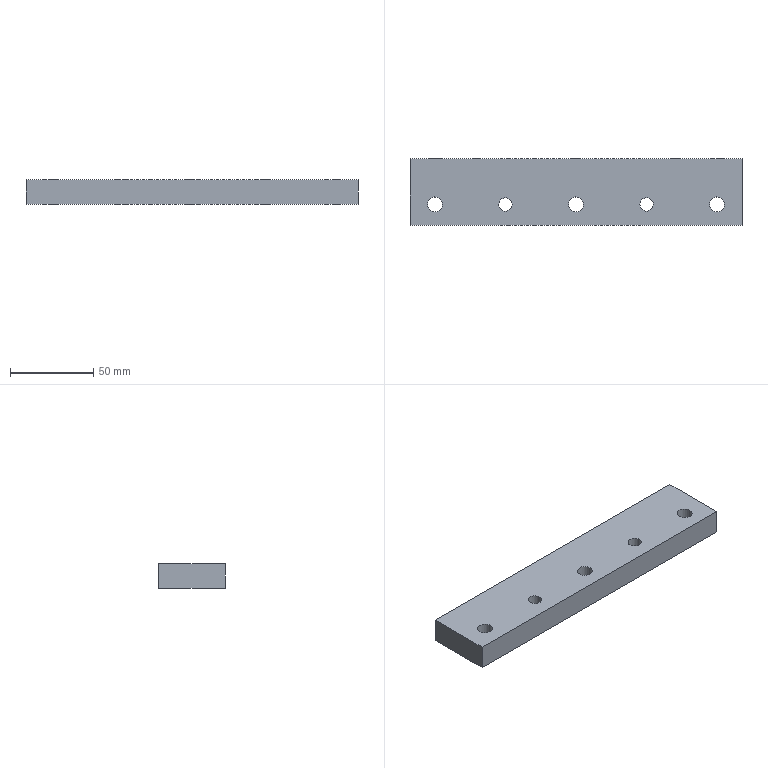Part | STEP file | SN10_002_007_SUPORTE | 1 solid | 21 faces | box 200 x 40 x 15 mm | volume 112375 mm3 | cylinder 10 | plane 6 | cone 5 | commonest cylinder face diameters 8 x4 4.917 x3 9 x3
STEP:
#1=CARTESIAN_POINT('',(0.,0.,0.));
#2=DIRECTION('',(0.,0.,1.));
#3=DIRECTION('',(1.,0.,0.));
#4=AXIS2_PLACEMENT_3D('',#1,#2,#3);
#5=CARTESIAN_POINT('',(-81.49,195.,59.418));
#6=VERTEX_POINT('',#5);
#7=CARTESIAN_POINT('',(-85.,195.,57.5));
#8=DIRECTION('',(0.,1.,0.));
#9=DIRECTION('',(1.,0.,0.));
#10=AXIS2_PLACEMENT_3D('',#7,#8,#9);
#11=CIRCLE('',#10,4.);
#12=CARTESIAN_POINT('',(-85.,193.268,57.5));
#13=DIRECTION('',(0.,1.,0.));
#14=DIRECTION('',(0.8776,0.,0.4794));
#15=AXIS2_PLACEMENT_3D('',#12,#13,#14);
#16=CONICAL_SURFACE('',#15,1.,1.047);
#17=CARTESIAN_POINT('',(-5.783,1.732));
#18=DIRECTION('',(1.,0.));
#19=VECTOR('',#18,1.);
#20=LINE('',#17,#19);
#21=(GEOMETRIC_REPRESENTATION_CONTEXT(2)PARAMETRIC_REPRESENTATION_CONTEXT()REPRESENTATION_CONTEXT('',''));
#22=DEFINITIONAL_REPRESENTATION('',(#20),#21);
#23=PCURVE('',#16,#22);
#24=CARTESIAN_POINT('',(-85.,214.9,57.5));
#25=DIRECTION('',(0.,-1.,0.));
#26=DIRECTION('',(0.8776,0.,0.4794));
#27=AXIS2_PLACEMENT_3D('',#24,#25,#26);
#28=CYLINDRICAL_SURFACE('',#27,4.);
#29=CARTESIAN_POINT('',(12.066,19.9));
#30=DIRECTION('',(-1.,0.));
#31=VECTOR('',#30,1.);
#32=LINE('',#29,#31);
#33=(GEOMETRIC_REPRESENTATION_CONTEXT(2)PARAMETRIC_REPRESENTATION_CONTEXT()REPRESENTATION_CONTEXT('',''));
#34=DEFINITIONAL_REPRESENTATION('',(#32),#33);
#35=PCURVE('',#28,#34);
#36=SURFACE_CURVE('',#11,(#23,#35),.PCURVE_S1.);
#37=EDGE_CURVE('',#6,#6,#36,.T.);
#38=ORIENTED_EDGE('',*,*,#37,.F.);
#39=CARTESIAN_POINT('',(-85.,192.691,57.5));
#40=VERTEX_POINT('',#39);
#41=CARTESIAN_POINT('',(-85.,192.691,57.5));
#42=CARTESIAN_POINT('',(-81.49,195.,59.418));
#43=B_SPLINE_CURVE_WITH_KNOTS('',1,(#41,#42),.UNSPECIFIED.,.F.,.F.,(2,2),(-1.155,3.464),.PIECEWISE_BEZIER_KNOTS.);
#44=CARTESIAN_POINT('',(0.,0.));
#45=DIRECTION('',(0.,1.));
#46=VECTOR('',#45,1.);
#47=LINE('',#44,#46);
#48=(GEOMETRIC_REPRESENTATION_CONTEXT(2)PARAMETRIC_REPRESENTATION_CONTEXT()REPRESENTATION_CONTEXT('',''));
#49=DEFINITIONAL_REPRESENTATION('',(#47),#48);
#50=PCURVE('',#16,#49);
#51=CARTESIAN_POINT('',(6.283,0.));
#52=DIRECTION('',(0.,1.));
#53=VECTOR('',#52,1.);
#54=LINE('',#51,#53);
#55=(GEOMETRIC_REPRESENTATION_CONTEXT(2)PARAMETRIC_REPRESENTATION_CONTEXT()REPRESENTATION_CONTEXT('',''));
#56=DEFINITIONAL_REPRESENTATION('',(#54),#55);
#57=PCURVE('',#16,#56);
#58=SEAM_CURVE('',#43,(#50,#57),.PCURVE_S1.);
#59=EDGE_CURVE('',#40,#6,#58,.T.);
#60=ORIENTED_EDGE('',*,*,#59,.F.);
#61=ORIENTED_EDGE('',*,*,#59,.T.);
#62=EDGE_LOOP('',(#38,#60,#61));
#63=FACE_BOUND('',#62,.F.);
#64=ADVANCED_FACE('',(#63),#16,.F.);
#65=CARTESIAN_POINT('',(-100.,215.,65.));
#66=VERTEX_POINT('',#65);
#67=CARTESIAN_POINT('',(100.,215.,65.));
#68=VERTEX_POINT('',#67);
#69=CARTESIAN_POINT('',(-100.,215.,65.));
#70=DIRECTION('',(1.,0.,0.));
#71=VECTOR('',#70,1.);
#72=LINE('',#69,#71);
#73=CARTESIAN_POINT('',(0.,175.,65.));
#74=DIRECTION('',(0.,0.,-1.));
#75=DIRECTION('',(-1.,0.,0.));
#76=AXIS2_PLACEMENT_3D('',#73,#74,#75);
#77=PLANE('',#76);
#78=CARTESIAN_POINT('',(100.,40.));
#79=DIRECTION('',(-1.,0.));
#80=VECTOR('',#79,1.);
#81=LINE('',#78,#80);
#82=(GEOMETRIC_REPRESENTATION_CONTEXT(2)PARAMETRIC_REPRESENTATION_CONTEXT()REPRESENTATION_CONTEXT('',''));
#83=DEFINITIONAL_REPRESENTATION('',(#81),#82);
#84=PCURVE('',#77,#83);
#85=CARTESIAN_POINT('',(0.,215.,65.));
#86=DIRECTION('',(0.,-1.,0.));
#87=DIRECTION('',(0.,0.,-1.));
#88=AXIS2_PLACEMENT_3D('',#85,#86,#87);
#89=PLANE('',#88);
#90=CARTESIAN_POINT('',(0.,-100.));
#91=DIRECTION('',(0.,1.));
#92=VECTOR('',#91,1.);
#93=LINE('',#90,#92);
#94=(GEOMETRIC_REPRESENTATION_CONTEXT(2)PARAMETRIC_REPRESENTATION_CONTEXT()REPRESENTATION_CONTEXT('',''));
#95=DEFINITIONAL_REPRESENTATION('',(#93),#94);
#96=PCURVE('',#89,#95);
#97=SURFACE_CURVE('',#72,(#84,#96),.PCURVE_S1.);
#98=EDGE_CURVE('',#66,#68,#97,.T.);
#99=ORIENTED_EDGE('',*,*,#98,.F.);
#100=CARTESIAN_POINT('',(-100.,175.,65.));
#101=VERTEX_POINT('',#100);
#102=CARTESIAN_POINT('',(-100.,175.,65.));
#103=DIRECTION('',(0.,1.,0.));
#104=VECTOR('',#103,1.);
#105=LINE('',#102,#104);
#106=CARTESIAN_POINT('',(100.,0.));
#107=DIRECTION('',(0.,1.));
#108=VECTOR('',#107,1.);
#109=LINE('',#106,#108);
#110=(GEOMETRIC_REPRESENTATION_CONTEXT(2)PARAMETRIC_REPRESENTATION_CONTEXT()REPRESENTATION_CONTEXT('',''));
#111=DEFINITIONAL_REPRESENTATION('',(#109),#110);
#112=PCURVE('',#77,#111);
#113=CARTESIAN_POINT('',(-100.,0.,0.));
#114=DIRECTION('',(1.,0.,0.));
#115=DIRECTION('',(0.,0.,-1.));
#116=AXIS2_PLACEMENT_3D('',#113,#114,#115);
#117=PLANE('',#116);
#118=CARTESIAN_POINT('',(-65.,175.));
#119=DIRECTION('',(0.,1.));
#120=VECTOR('',#119,1.);
#121=LINE('',#118,#120);
#122=(GEOMETRIC_REPRESENTATION_CONTEXT(2)PARAMETRIC_REPRESENTATION_CONTEXT()REPRESENTATION_CONTEXT('',''));
#123=DEFINITIONAL_REPRESENTATION('',(#121),#122);
#124=PCURVE('',#117,#123);
#125=SURFACE_CURVE('',#105,(#112,#124),.PCURVE_S1.);
#126=EDGE_CURVE('',#101,#66,#125,.T.);
#127=ORIENTED_EDGE('',*,*,#126,.F.);
#128=CARTESIAN_POINT('',(100.,175.,65.));
#129=VERTEX_POINT('',#128);
#130=CARTESIAN_POINT('',(-100.,175.,65.));
#131=DIRECTION('',(1.,0.,0.));
#132=VECTOR('',#131,1.);
#133=LINE('',#130,#132);
#134=CARTESIAN_POINT('',(100.,0.));
#135=DIRECTION('',(-1.,0.));
#136=VECTOR('',#135,1.);
#137=LINE('',#134,#136);
#138=(GEOMETRIC_REPRESENTATION_CONTEXT(2)PARAMETRIC_REPRESENTATION_CONTEXT()REPRESENTATION_CONTEXT('',''));
#139=DEFINITIONAL_REPRESENTATION('',(#137),#138);
#140=PCURVE('',#77,#139);
#141=CARTESIAN_POINT('',(0.,175.,50.));
#142=DIRECTION('',(0.,1.,0.));
#143=DIRECTION('',(0.,0.,1.));
#144=AXIS2_PLACEMENT_3D('',#141,#142,#143);
#145=PLANE('',#144);
#146=CARTESIAN_POINT('',(15.,-100.));
#147=DIRECTION('',(0.,1.));
#148=VECTOR('',#147,1.);
#149=LINE('',#146,#148);
#150=(GEOMETRIC_REPRESENTATION_CONTEXT(2)PARAMETRIC_REPRESENTATION_CONTEXT()REPRESENTATION_CONTEXT('',''));
#151=DEFINITIONAL_REPRESENTATION('',(#149),#150);
#152=PCURVE('',#145,#151);
#153=SURFACE_CURVE('',#133,(#140,#152),.PCURVE_S1.);
#154=EDGE_CURVE('',#101,#129,#153,.T.);
#155=ORIENTED_EDGE('',*,*,#154,.T.);
#156=CARTESIAN_POINT('',(100.,175.,65.));
#157=DIRECTION('',(0.,1.,0.));
#158=VECTOR('',#157,1.);
#159=LINE('',#156,#158);
#160=CARTESIAN_POINT('',(-100.,0.));
#161=DIRECTION('',(0.,1.));
#162=VECTOR('',#161,1.);
#163=LINE('',#160,#162);
#164=(GEOMETRIC_REPRESENTATION_CONTEXT(2)PARAMETRIC_REPRESENTATION_CONTEXT()REPRESENTATION_CONTEXT('',''));
#165=DEFINITIONAL_REPRESENTATION('',(#163),#164);
#166=PCURVE('',#77,#165);
#167=CARTESIAN_POINT('',(100.,0.,0.));
#168=DIRECTION('',(1.,0.,0.));
#169=DIRECTION('',(0.,0.,-1.));
#170=AXIS2_PLACEMENT_3D('',#167,#168,#169);
#171=PLANE('',#170);
#172=CARTESIAN_POINT('',(-65.,175.));
#173=DIRECTION('',(0.,1.));
#174=VECTOR('',#173,1.);
#175=LINE('',#172,#174);
#176=(GEOMETRIC_REPRESENTATION_CONTEXT(2)PARAMETRIC_REPRESENTATION_CONTEXT()REPRESENTATION_CONTEXT('',''));
#177=DEFINITIONAL_REPRESENTATION('',(#175),#176);
#178=PCURVE('',#171,#177);
#179=SURFACE_CURVE('',#159,(#166,#178),.PCURVE_S1.);
#180=EDGE_CURVE('',#129,#68,#179,.T.);
#181=ORIENTED_EDGE('',*,*,#180,.T.);
#182=EDGE_LOOP('',(#99,#127,#155,#181));
#183=FACE_BOUND('',#182,.T.);
#184=CARTESIAN_POINT('',(38.99,189.418,65.));
#185=VERTEX_POINT('',#184);
#186=CARTESIAN_POINT('',(42.5,187.5,65.));
#187=DIRECTION('',(0.,0.,-1.));
#188=DIRECTION('',(1.,0.,0.));
#189=AXIS2_PLACEMENT_3D('',#186,#187,#188);
#190=CIRCLE('',#189,4.);
#191=CARTESIAN_POINT('',(-42.5,12.5));
#192=DIRECTION('',(-1.,0.));
#193=AXIS2_PLACEMENT_2D('',#191,#192);
#194=CIRCLE('',#193,4.);
#195=(GEOMETRIC_REPRESENTATION_CONTEXT(2)PARAMETRIC_REPRESENTATION_CONTEXT()REPRESENTATION_CONTEXT('',''));
#196=DEFINITIONAL_REPRESENTATION('',(#194),#195);
#197=PCURVE('',#77,#196);
#198=CARTESIAN_POINT('',(42.5,187.5,64.9));
#199=DIRECTION('',(0.,0.,-1.));
#200=DIRECTION('',(0.8776,-0.4794,0.));
#201=AXIS2_PLACEMENT_3D('',#198,#199,#200);
#202=CYLINDRICAL_SURFACE('',#201,4.);
#203=CARTESIAN_POINT('',(-0.5,-0.1));
#204=DIRECTION('',(1.,0.));
#205=VECTOR('',#204,1.);
#206=LINE('',#203,#205);
#207=(GEOMETRIC_REPRESENTATION_CONTEXT(2)PARAMETRIC_REPRESENTATION_CONTEXT()REPRESENTATION_CONTEXT('',''));
#208=DEFINITIONAL_REPRESENTATION('',(#206),#207);
#209=PCURVE('',#202,#208);
#210=SURFACE_CURVE('',#190,(#197,#209),.PCURVE_S1.);
#211=EDGE_CURVE('',#185,#185,#210,.T.);
#212=ORIENTED_EDGE('',*,*,#211,.T.);
#213=EDGE_LOOP('',(#212));
#214=FACE_BOUND('',#213,.T.);
#215=CARTESIAN_POINT('',(-46.01,189.418,65.));
#216=VERTEX_POINT('',#215);
#217=CARTESIAN_POINT('',(-42.5,187.5,65.));
#218=DIRECTION('',(0.,0.,-1.));
#219=DIRECTION('',(1.,0.,0.));
#220=AXIS2_PLACEMENT_3D('',#217,#218,#219);
#221=CIRCLE('',#220,4.);
#222=CARTESIAN_POINT('',(42.5,12.5));
#223=DIRECTION('',(-1.,0.));
#224=AXIS2_PLACEMENT_2D('',#222,#223);
#225=CIRCLE('',#224,4.);
#226=(GEOMETRIC_REPRESENTATION_CONTEXT(2)PARAMETRIC_REPRESENTATION_CONTEXT()REPRESENTATION_CONTEXT('',''));
#227=DEFINITIONAL_REPRESENTATION('',(#225),#226);
#228=PCURVE('',#77,#227);
#229=CARTESIAN_POINT('',(-42.5,187.5,64.9));
#230=DIRECTION('',(0.,0.,-1.));
#231=DIRECTION('',(0.8776,-0.4794,0.));
#232=AXIS2_PLACEMENT_3D('',#229,#230,#231);
#233=CYLINDRICAL_SURFACE('',#232,4.);
#234=CARTESIAN_POINT('',(-0.5,-0.1));
#235=DIRECTION('',(1.,0.));
#236=VECTOR('',#235,1.);
#237=LINE('',#234,#236);
#238=(GEOMETRIC_REPRESENTATION_CONTEXT(2)PARAMETRIC_REPRESENTATION_CONTEXT()REPRESENTATION_CONTEXT('',''));
#239=DEFINITIONAL_REPRESENTATION('',(#237),#238);
#240=PCURVE('',#233,#239);
#241=SURFACE_CURVE('',#221,(#228,#240),.PCURVE_S1.);
#242=EDGE_CURVE('',#216,#216,#241,.T.);
#243=ORIENTED_EDGE('',*,*,#242,.T.);
#244=EDGE_LOOP('',(#243));
#245=FACE_BOUND('',#244,.T.);
#246=CARTESIAN_POINT('',(-88.949,189.657,65.));
#247=VERTEX_POINT('',#246);
#248=CARTESIAN_POINT('',(-85.,187.5,65.));
#249=DIRECTION('',(0.,0.,-1.));
#250=DIRECTION('',(1.,0.,0.));
#251=AXIS2_PLACEMENT_3D('',#248,#249,#250);
#252=CIRCLE('',#251,4.5);
#253=CARTESIAN_POINT('',(85.,12.5));
#254=DIRECTION('',(-1.,0.));
#255=AXIS2_PLACEMENT_2D('',#253,#254);
#256=CIRCLE('',#255,4.5);
#257=(GEOMETRIC_REPRESENTATION_CONTEXT(2)PARAMETRIC_REPRESENTATION_CONTEXT()REPRESENTATION_CONTEXT('',''));
#258=DEFINITIONAL_REPRESENTATION('',(#256),#257);
#259=PCURVE('',#77,#258);
#260=CARTESIAN_POINT('',(-85.,187.5,64.9));
#261=DIRECTION('',(0.,0.,-1.));
#262=DIRECTION('',(0.8776,-0.4794,0.));
#263=AXIS2_PLACEMENT_3D('',#260,#261,#262);
#264=CYLINDRICAL_SURFACE('',#263,4.5);
#265=CARTESIAN_POINT('',(-0.5,-0.1));
#266=DIRECTION('',(1.,0.));
#267=VECTOR('',#266,1.);
#268=LINE('',#265,#267);
#269=(GEOMETRIC_REPRESENTATION_CONTEXT(2)PARAMETRIC_REPRESENTATION_CONTEXT()REPRESENTATION_CONTEXT('',''));
#270=DEFINITIONAL_REPRESENTATION('',(#268),#269);
#271=PCURVE('',#264,#270);
#272=SURFACE_CURVE('',#252,(#259,#271),.PCURVE_S1.);
#273=EDGE_CURVE('',#247,#247,#272,.T.);
#274=ORIENTED_EDGE('',*,*,#273,.T.);
#275=EDGE_LOOP('',(#274));
#276=FACE_BOUND('',#275,.T.);
#277=CARTESIAN_POINT('',(-3.949,189.657,65.));
#278=VERTEX_POINT('',#277);
#279=CARTESIAN_POINT('',(0.,187.5,65.));
#280=DIRECTION('',(0.,0.,-1.));
#281=DIRECTION('',(1.,0.,0.));
#282=AXIS2_PLACEMENT_3D('',#279,#280,#281);
#283=CIRCLE('',#282,4.5);
#284=CARTESIAN_POINT('',(0.,12.5));
#285=DIRECTION('',(-1.,0.));
#286=AXIS2_PLACEMENT_2D('',#284,#285);
#287=CIRCLE('',#286,4.5);
#288=(GEOMETRIC_REPRESENTATION_CONTEXT(2)PARAMETRIC_REPRESENTATION_CONTEXT()REPRESENTATION_CONTEXT('',''));
#289=DEFINITIONAL_REPRESENTATION('',(#287),#288);
#290=PCURVE('',#77,#289);
#291=CARTESIAN_POINT('',(0.,187.5,64.9));
#292=DIRECTION('',(0.,0.,-1.));
#293=DIRECTION('',(0.8776,-0.4794,0.));
#294=AXIS2_PLACEMENT_3D('',#291,#292,#293);
#295=CYLINDRICAL_SURFACE('',#294,4.5);
#296=CARTESIAN_POINT('',(-0.5,-0.1));
#297=DIRECTION('',(1.,0.));
#298=VECTOR('',#297,1.);
#299=LINE('',#296,#298);
#300=(GEOMETRIC_REPRESENTATION_CONTEXT(2)PARAMETRIC_REPRESENTATION_CONTEXT()REPRESENTATION_CONTEXT('',''));
#301=DEFINITIONAL_REPRESENTATION('',(#299),#300);
#302=PCURVE('',#295,#301);
#303=SURFACE_CURVE('',#283,(#290,#302),.PCURVE_S1.);
#304=EDGE_CURVE('',#278,#278,#303,.T.);
#305=ORIENTED_EDGE('',*,*,#304,.T.);
#306=EDGE_LOOP('',(#305));
#307=FACE_BOUND('',#306,.T.);
#308=CARTESIAN_POINT('',(81.051,189.657,65.));
#309=VERTEX_POINT('',#308);
#310=CARTESIAN_POINT('',(85.,187.5,65.));
#311=DIRECTION('',(0.,0.,-1.));
#312=DIRECTION('',(1.,0.,0.));
#313=AXIS2_PLACEMENT_3D('',#310,#311,#312);
#314=CIRCLE('',#313,4.5);
#315=CARTESIAN_POINT('',(-85.,12.5));
#316=DIRECTION('',(-1.,0.));
#317=AXIS2_PLACEMENT_2D('',#315,#316);
#318=CIRCLE('',#317,4.5);
#319=(GEOMETRIC_REPRESENTATION_CONTEXT(2)PARAMETRIC_REPRESENTATION_CONTEXT()REPRESENTATION_CONTEXT('',''));
#320=DEFINITIONAL_REPRESENTATION('',(#318),#319);
#321=PCURVE('',#77,#320);
#322=CARTESIAN_POINT('',(85.,187.5,64.9));
#323=DIRECTION('',(0.,0.,-1.));
#324=DIRECTION('',(0.8776,-0.4794,0.));
#325=AXIS2_PLACEMENT_3D('',#322,#323,#324);
#326=CYLINDRICAL_SURFACE('',#325,4.5);
#327=CARTESIAN_POINT('',(-0.5,-0.1));
#328=DIRECTION('',(1.,0.));
#329=VECTOR('',#328,1.);
#330=LINE('',#327,#329);
#331=(GEOMETRIC_REPRESENTATION_CONTEXT(2)PARAMETRIC_REPRESENTATION_CONTEXT()REPRESENTATION_CONTEXT('',''));
#332=DEFINITIONAL_REPRESENTATION('',(#330),#331);
#333=PCURVE('',#326,#332);
#334=SURFACE_CURVE('',#314,(#321,#333),.PCURVE_S1.);
#335=EDGE_CURVE('',#309,#309,#334,.T.);
#336=ORIENTED_EDGE('',*,*,#335,.T.);
#337=EDGE_LOOP('',(#336));
#338=FACE_BOUND('',#337,.T.);
#339=ADVANCED_FACE('',(#183,#214,#245,#276,#307,#338),#77,.F.);
#340=CARTESIAN_POINT('',(-100.,215.,50.));
#341=VERTEX_POINT('',#340);
#342=CARTESIAN_POINT('',(-100.,215.,65.));
#343=DIRECTION('',(0.,0.,-1.));
#344=VECTOR('',#343,1.);
#345=LINE('',#342,#344);
#346=CARTESIAN_POINT('',(-65.,215.));
#347=DIRECTION('',(1.,0.));
#348=VECTOR('',#347,1.);
#349=LINE('',#346,#348);
#350=(GEOMETRIC_REPRESENTATION_CONTEXT(2)PARAMETRIC_REPRESENTATION_CONTEXT()REPRESENTATION_CONTEXT('',''));
#351=DEFINITIONAL_REPRESENTATION('',(#349),#350);
#352=PCURVE('',#117,#351);
#353=CARTESIAN_POINT('',(0.,-100.));
#354=DIRECTION('',(1.,0.));
#355=VECTOR('',#354,1.);
#356=LINE('',#353,#355);
#357=(GEOMETRIC_REPRESENTATION_CONTEXT(2)PARAMETRIC_REPRESENTATION_CONTEXT()REPRESENTATION_CONTEXT('',''));
#358=DEFINITIONAL_REPRESENTATION('',(#356),#357);
#359=PCURVE('',#89,#358);
#360=SURFACE_CURVE('',#345,(#352,#359),.PCURVE_S1.);
#361=EDGE_CURVE('',#66,#341,#360,.T.);
#362=ORIENTED_EDGE('',*,*,#361,.T.);
#363=CARTESIAN_POINT('',(-100.,175.,50.));
#364=VERTEX_POINT('',#363);
#365=CARTESIAN_POINT('',(-100.,215.,50.));
#366=DIRECTION('',(0.,-1.,0.));
#367=VECTOR('',#366,1.);
#368=LINE('',#365,#367);
#369=CARTESIAN_POINT('',(-50.,215.));
#370=DIRECTION('',(0.,-1.));
#371=VECTOR('',#370,1.);
#372=LINE('',#369,#371);
#373=(GEOMETRIC_REPRESENTATION_CONTEXT(2)PARAMETRIC_REPRESENTATION_CONTEXT()REPRESENTATION_CONTEXT('',''));
#374=DEFINITIONAL_REPRESENTATION('',(#372),#373);
#375=PCURVE('',#117,#374);
#376=CARTESIAN_POINT('',(0.,215.,50.));
#377=DIRECTION('',(0.,0.,1.));
#378=DIRECTION('',(1.,0.,0.));
#379=AXIS2_PLACEMENT_3D('',#376,#377,#378);
#380=PLANE('',#379);
#381=CARTESIAN_POINT('',(-100.,0.));
#382=DIRECTION('',(0.,-1.));
#383=VECTOR('',#382,1.);
#384=LINE('',#381,#383);
#385=(GEOMETRIC_REPRESENTATION_CONTEXT(2)PARAMETRIC_REPRESENTATION_CONTEXT()REPRESENTATION_CONTEXT('',''));
#386=DEFINITIONAL_REPRESENTATION('',(#384),#385);
#387=PCURVE('',#380,#386);
#388=SURFACE_CURVE('',#368,(#375,#387),.PCURVE_S1.);
#389=EDGE_CURVE('',#341,#364,#388,.T.);
#390=ORIENTED_EDGE('',*,*,#389,.T.);
#391=CARTESIAN_POINT('',(-100.,175.,50.));
#392=DIRECTION('',(0.,0.,1.));
#393=VECTOR('',#392,1.);
#394=LINE('',#391,#393);
#395=CARTESIAN_POINT('',(-50.,175.));
#396=DIRECTION('',(-1.,0.));
#397=VECTOR('',#396,1.);
#398=LINE('',#395,#397);
#399=(GEOMETRIC_REPRESENTATION_CONTEXT(2)PARAMETRIC_REPRESENTATION_CONTEXT()REPRESENTATION_CONTEXT('',''));
#400=DEFINITIONAL_REPRESENTATION('',(#398),#399);
#401=PCURVE('',#117,#400);
#402=CARTESIAN_POINT('',(0.,-100.));
#403=DIRECTION('',(1.,0.));
#404=VECTOR('',#403,1.);
#405=LINE('',#402,#404);
#406=(GEOMETRIC_REPRESENTATION_CONTEXT(2)PARAMETRIC_REPRESENTATION_CONTEXT()REPRESENTATION_CONTEXT('',''));
#407=DEFINITIONAL_REPRESENTATION('',(#405),#406);
#408=PCURVE('',#145,#407);
#409=SURFACE_CURVE('',#394,(#401,#408),.PCURVE_S1.);
#410=EDGE_CURVE('',#364,#101,#409,.T.);
#411=ORIENTED_EDGE('',*,*,#410,.T.);
#412=ORIENTED_EDGE('',*,*,#126,.T.);
#413=EDGE_LOOP('',(#362,#390,#411,#412));
#414=FACE_BOUND('',#413,.T.);
#415=ADVANCED_FACE('',(#414),#117,.F.);
#416=CARTESIAN_POINT('',(81.49,215.,55.582));
#417=VERTEX_POINT('',#416);
#418=CARTESIAN_POINT('',(85.,215.,57.5));
#419=DIRECTION('',(0.,-1.,0.));
#420=DIRECTION('',(1.,0.,0.));
#421=AXIS2_PLACEMENT_3D('',#418,#419,#420);
#422=CIRCLE('',#421,4.);
#423=CARTESIAN_POINT('',(85.,214.9,57.5));
#424=DIRECTION('',(0.,-1.,0.));
#425=DIRECTION('',(0.8776,0.,0.4794));
#426=AXIS2_PLACEMENT_3D('',#423,#424,#425);
#427=CYLINDRICAL_SURFACE('',#426,4.);
#428=CARTESIAN_POINT('',(-0.5,-0.1));
#429=DIRECTION('',(1.,0.));
#430=VECTOR('',#429,1.);
#431=LINE('',#428,#430);
#432=(GEOMETRIC_REPRESENTATION_CONTEXT(2)PARAMETRIC_REPRESENTATION_CONTEXT()REPRESENTATION_CONTEXT('',''));
#433=DEFINITIONAL_REPRESENTATION('',(#431),#432);
#434=PCURVE('',#427,#433);
#435=CARTESIAN_POINT('',(7.5,85.));
#436=DIRECTION('',(0.,1.));
#437=AXIS2_PLACEMENT_2D('',#435,#436);
#438=CIRCLE('',#437,4.);
#439=(GEOMETRIC_REPRESENTATION_CONTEXT(2)PARAMETRIC_REPRESENTATION_CONTEXT()REPRESENTATION_CONTEXT('',''));
#440=DEFINITIONAL_REPRESENTATION('',(#438),#439);
#441=PCURVE('',#89,#440);
#442=SURFACE_CURVE('',#422,(#434,#441),.PCURVE_S1.);
#443=EDGE_CURVE('',#417,#417,#442,.T.);
#444=ORIENTED_EDGE('',*,*,#443,.T.);
#445=CARTESIAN_POINT('',(81.49,195.,55.582));
#446=VERTEX_POINT('',#445);
#447=CARTESIAN_POINT('',(81.49,215.,55.582));
#448=CARTESIAN_POINT('',(81.49,195.,55.582));
#449=B_SPLINE_CURVE_WITH_KNOTS('',1,(#447,#448),.UNSPECIFIED.,.F.,.F.,(2,2),(-0.1,19.9),.PIECEWISE_BEZIER_KNOTS.);
#450=CARTESIAN_POINT('',(9.425,0.));
#451=DIRECTION('',(0.,1.));
#452=VECTOR('',#451,1.);
#453=LINE('',#450,#452);
#454=(GEOMETRIC_REPRESENTATION_CONTEXT(2)PARAMETRIC_REPRESENTATION_CONTEXT()REPRESENTATION_CONTEXT('',''));
#455=DEFINITIONAL_REPRESENTATION('',(#453),#454);
#456=PCURVE('',#427,#455);
#457=CARTESIAN_POINT('',(3.142,0.));
#458=DIRECTION('',(0.,1.));
#459=VECTOR('',#458,1.);
#460=LINE('',#457,#459);
#461=(GEOMETRIC_REPRESENTATION_CONTEXT(2)PARAMETRIC_REPRESENTATION_CONTEXT()REPRESENTATION_CONTEXT('',''));
#462=DEFINITIONAL_REPRESENTATION('',(#460),#461);
#463=PCURVE('',#427,#462);
#464=SEAM_CURVE('',#449,(#456,#463),.PCURVE_S1.);
#465=EDGE_CURVE('',#417,#446,#464,.T.);
#466=ORIENTED_EDGE('',*,*,#465,.T.);
#467=CARTESIAN_POINT('',(85.,195.,57.5));
#468=DIRECTION('',(0.,-1.,0.));
#469=DIRECTION('',(1.,0.,0.));
#470=AXIS2_PLACEMENT_3D('',#467,#468,#469);
#471=CIRCLE('',#470,4.);
#472=CARTESIAN_POINT('',(-0.5,19.9));
#473=DIRECTION('',(1.,0.));
#474=VECTOR('',#473,1.);
#475=LINE('',#472,#474);
#476=(GEOMETRIC_REPRESENTATION_CONTEXT(2)PARAMETRIC_REPRESENTATION_CONTEXT()REPRESENTATION_CONTEXT('',''));
#477=DEFINITIONAL_REPRESENTATION('',(#475),#476);
#478=PCURVE('',#427,#477);
#479=CARTESIAN_POINT('',(85.,193.268,57.5));
#480=DIRECTION('',(0.,1.,0.));
#481=DIRECTION('',(0.8776,0.,0.4794));
#482=AXIS2_PLACEMENT_3D('',#479,#480,#481);
#483=CONICAL_SURFACE('',#482,1.,1.047);
#484=CARTESIAN_POINT('',(13.066,1.732));
#485=DIRECTION('',(-1.,0.));
#486=VECTOR('',#485,1.);
#487=LINE('',#484,#486);
#488=(GEOMETRIC_REPRESENTATION_CONTEXT(2)PARAMETRIC_REPRESENTATION_CONTEXT()REPRESENTATION_CONTEXT('',''));
#489=DEFINITIONAL_REPRESENTATION('',(#487),#488);
#490=PCURVE('',#483,#489);
#491=SURFACE_CURVE('',#471,(#478,#490),.PCURVE_S1.);
#492=EDGE_CURVE('',#446,#446,#491,.T.);
#493=ORIENTED_EDGE('',*,*,#492,.F.);
#494=ORIENTED_EDGE('',*,*,#465,.F.);
#495=EDGE_LOOP('',(#444,#466,#493,#494));
#496=FACE_BOUND('',#495,.F.);
#497=ADVANCED_FACE('',(#496),#427,.F.);
#498=CARTESIAN_POINT('',(-62.158,215.,56.321));
#499=VERTEX_POINT('',#498);
#500=CARTESIAN_POINT('',(-60.,215.,57.5));
#501=DIRECTION('',(0.,-1.,0.));
#502=DIRECTION('',(1.,0.,0.));
#503=AXIS2_PLACEMENT_3D('',#500,#501,#502);
#504=CIRCLE('',#503,2.458);
#505=CARTESIAN_POINT('',(-60.,214.9,57.5));
#506=DIRECTION('',(0.,-1.,0.));
#507=DIRECTION('',(0.8776,0.,0.4794));
#508=AXIS2_PLACEMENT_3D('',#505,#506,#507);
#509=CYLINDRICAL_SURFACE('',#508,2.458);
#510=CARTESIAN_POINT('',(-0.5,-0.1));
#511=DIRECTION('',(1.,0.));
#512=VECTOR('',#511,1.);
#513=LINE('',#510,#512);
#514=(GEOMETRIC_REPRESENTATION_CONTEXT(2)PARAMETRIC_REPRESENTATION_CONTEXT()REPRESENTATION_CONTEXT('',''));
#515=DEFINITIONAL_REPRESENTATION('',(#513),#514);
#516=PCURVE('',#509,#515);
#517=CARTESIAN_POINT('',(7.5,-60.));
#518=DIRECTION('',(0.,1.));
#519=AXIS2_PLACEMENT_2D('',#517,#518);
#520=CIRCLE('',#519,2.458);
#521=(GEOMETRIC_REPRESENTATION_CONTEXT(2)PARAMETRIC_REPRESENTATION_CONTEXT()REPRESENTATION_CONTEXT('',''));
#522=DEFINITIONAL_REPRESENTATION('',(#520),#521);
#523=PCURVE('',#89,#522);
#524=SURFACE_CURVE('',#504,(#516,#523),.PCURVE_S1.);
#525=EDGE_CURVE('',#499,#499,#524,.T.);
#526=ORIENTED_EDGE('',*,*,#525,.T.);
#527=CARTESIAN_POINT('',(-62.158,195.,56.321));
#528=VERTEX_POINT('',#527);
#529=CARTESIAN_POINT('',(-62.158,215.,56.321));
#530=CARTESIAN_POINT('',(-62.158,195.,56.321));
#531=B_SPLINE_CURVE_WITH_KNOTS('',1,(#529,#530),.UNSPECIFIED.,.F.,.F.,(2,2),(-0.1,19.9),.PIECEWISE_BEZIER_KNOTS.);
#532=CARTESIAN_POINT('',(9.425,0.));
#533=DIRECTION('',(0.,1.));
#534=VECTOR('',#533,1.);
#535=LINE('',#532,#534);
#536=(GEOMETRIC_REPRESENTATION_CONTEXT(2)PARAMETRIC_REPRESENTATION_CONTEXT()REPRESENTATION_CONTEXT('',''));
#537=DEFINITIONAL_REPRESENTATION('',(#535),#536);
#538=PCURVE('',#509,#537);
#539=CARTESIAN_POINT('',(3.142,0.));
#540=DIRECTION('',(0.,1.));
#541=VECTOR('',#540,1.);
#542=LINE('',#539,#541);
#543=(GEOMETRIC_REPRESENTATION_CONTEXT(2)PARAMETRIC_REPRESENTATION_CONTEXT()REPRESENTATION_CONTEXT('',''));
#544=DEFINITIONAL_REPRESENTATION('',(#542),#543);
#545=PCURVE('',#509,#544);
#546=SEAM_CURVE('',#531,(#538,#545),.PCURVE_S1.);
#547=EDGE_CURVE('',#499,#528,#546,.T.);
#548=ORIENTED_EDGE('',*,*,#547,.T.);
#549=CARTESIAN_POINT('',(-60.,195.,57.5));
#550=DIRECTION('',(0.,-1.,0.));
#551=DIRECTION('',(1.,0.,0.));
#552=AXIS2_PLACEMENT_3D('',#549,#550,#551);
#553=CIRCLE('',#552,2.458);
#554=CARTESIAN_POINT('',(-0.5,19.9));
#555=DIRECTION('',(1.,0.));
#556=VECTOR('',#555,1.);
#557=LINE('',#554,#556);
#558=(GEOMETRIC_REPRESENTATION_CONTEXT(2)PARAMETRIC_REPRESENTATION_CONTEXT()REPRESENTATION_CONTEXT('',''));
#559=DEFINITIONAL_REPRESENTATION('',(#557),#558);
#560=PCURVE('',#509,#559);
#561=CARTESIAN_POINT('',(-60.,194.158,57.5));
#562=DIRECTION('',(0.,1.,0.));
#563=DIRECTION('',(0.8776,0.,0.4794));
#564=AXIS2_PLACEMENT_3D('',#561,#562,#563);
#565=CONICAL_SURFACE('',#564,1.,1.047);
#566=CARTESIAN_POINT('',(13.066,0.8421));
#567=DIRECTION('',(-1.,0.));
#568=VECTOR('',#567,1.);
#569=LINE('',#566,#568);
#570=(GEOMETRIC_REPRESENTATION_CONTEXT(2)PARAMETRIC_REPRESENTATION_CONTEXT()REPRESENTATION_CONTEXT('',''));
#571=DEFINITIONAL_REPRESENTATION('',(#569),#570);
#572=PCURVE('',#565,#571);
#573=SURFACE_CURVE('',#553,(#560,#572),.PCURVE_S1.);
#574=EDGE_CURVE('',#528,#528,#573,.T.);
#575=ORIENTED_EDGE('',*,*,#574,.F.);
#576=ORIENTED_EDGE('',*,*,#547,.F.);
#577=EDGE_LOOP('',(#526,#548,#575,#576));
#578=FACE_BOUND('',#577,.F.);
#579=ADVANCED_FACE('',(#578),#509,.F.);
#580=CARTESIAN_POINT('',(-2.158,215.,56.321));
#581=VERTEX_POINT('',#580);
#582=CARTESIAN_POINT('',(0.,215.,57.5));
#583=DIRECTION('',(0.,-1.,0.));
#584=DIRECTION('',(1.,0.,0.));
#585=AXIS2_PLACEMENT_3D('',#582,#583,#584);
#586=CIRCLE('',#585,2.458);
#587=CARTESIAN_POINT('',(0.,214.9,57.5));
#588=DIRECTION('',(0.,-1.,0.));
#589=DIRECTION('',(0.8776,0.,0.4794));
#590=AXIS2_PLACEMENT_3D('',#587,#588,#589);
#591=CYLINDRICAL_SURFACE('',#590,2.458);
#592=CARTESIAN_POINT('',(-0.5,-0.1));
#593=DIRECTION('',(1.,0.));
#594=VECTOR('',#593,1.);
#595=LINE('',#592,#594);
#596=(GEOMETRIC_REPRESENTATION_CONTEXT(2)PARAMETRIC_REPRESENTATION_CONTEXT()REPRESENTATION_CONTEXT('',''));
#597=DEFINITIONAL_REPRESENTATION('',(#595),#596);
#598=PCURVE('',#591,#597);
#599=CARTESIAN_POINT('',(7.5,0.));
#600=DIRECTION('',(0.,1.));
#601=AXIS2_PLACEMENT_2D('',#599,#600);
#602=CIRCLE('',#601,2.458);
#603=(GEOMETRIC_REPRESENTATION_CONTEXT(2)PARAMETRIC_REPRESENTATION_CONTEXT()REPRESENTATION_CONTEXT('',''));
#604=DEFINITIONAL_REPRESENTATION('',(#602),#603);
#605=PCURVE('',#89,#604);
#606=SURFACE_CURVE('',#586,(#598,#605),.PCURVE_S1.);
#607=EDGE_CURVE('',#581,#581,#606,.T.);
#608=ORIENTED_EDGE('',*,*,#607,.T.);
#609=CARTESIAN_POINT('',(-2.158,195.,56.321));
#610=VERTEX_POINT('',#609);
#611=CARTESIAN_POINT('',(-2.158,215.,56.321));
#612=CARTESIAN_POINT('',(-2.158,195.,56.321));
#613=B_SPLINE_CURVE_WITH_KNOTS('',1,(#611,#612),.UNSPECIFIED.,.F.,.F.,(2,2),(-0.1,19.9),.PIECEWISE_BEZIER_KNOTS.);
#614=CARTESIAN_POINT('',(9.425,0.));
#615=DIRECTION('',(0.,1.));
#616=VECTOR('',#615,1.);
#617=LINE('',#614,#616);
#618=(GEOMETRIC_REPRESENTATION_CONTEXT(2)PARAMETRIC_REPRESENTATION_CONTEXT()REPRESENTATION_CONTEXT('',''));
#619=DEFINITIONAL_REPRESENTATION('',(#617),#618);
#620=PCURVE('',#591,#619);
#621=CARTESIAN_POINT('',(3.142,0.));
#622=DIRECTION('',(0.,1.));
#623=VECTOR('',#622,1.);
#624=LINE('',#621,#623);
#625=(GEOMETRIC_REPRESENTATION_CONTEXT(2)PARAMETRIC_REPRESENTATION_CONTEXT()REPRESENTATION_CONTEXT('',''));
#626=DEFINITIONAL_REPRESENTATION('',(#624),#625);
#627=PCURVE('',#591,#626);
#628=SEAM_CURVE('',#613,(#620,#627),.PCURVE_S1.);
#629=EDGE_CURVE('',#581,#610,#628,.T.);
#630=ORIENTED_EDGE('',*,*,#629,.T.);
#631=CARTESIAN_POINT('',(0.,195.,57.5));
#632=DIRECTION('',(0.,-1.,0.));
#633=DIRECTION('',(1.,0.,0.));
#634=AXIS2_PLACEMENT_3D('',#631,#632,#633);
#635=CIRCLE('',#634,2.458);
#636=CARTESIAN_POINT('',(-0.5,19.9));
#637=DIRECTION('',(1.,0.));
#638=VECTOR('',#637,1.);
#639=LINE('',#636,#638);
#640=(GEOMETRIC_REPRESENTATION_CONTEXT(2)PARAMETRIC_REPRESENTATION_CONTEXT()REPRESENTATION_CONTEXT('',''));
#641=DEFINITIONAL_REPRESENTATION('',(#639),#640);
#642=PCURVE('',#591,#641);
#643=CARTESIAN_POINT('',(0.,194.158,57.5));
#644=DIRECTION('',(0.,1.,0.));
#645=DIRECTION('',(0.8776,0.,0.4794));
#646=AXIS2_PLACEMENT_3D('',#643,#644,#645);
#647=CONICAL_SURFACE('',#646,1.,1.047);
#648=CARTESIAN_POINT('',(13.066,0.8421));
#649=DIRECTION('',(-1.,0.));
#650=VECTOR('',#649,1.);
#651=LINE('',#648,#650);
#652=(GEOMETRIC_REPRESENTATION_CONTEXT(2)PARAMETRIC_REPRESENTATION_CONTEXT()REPRESENTATION_CONTEXT('',''));
#653=DEFINITIONAL_REPRESENTATION('',(#651),#652);
#654=PCURVE('',#647,#653);
#655=SURFACE_CURVE('',#635,(#642,#654),.PCURVE_S1.);
#656=EDGE_CURVE('',#610,#610,#655,.T.);
#657=ORIENTED_EDGE('',*,*,#656,.F.);
#658=ORIENTED_EDGE('',*,*,#629,.F.);
#659=EDGE_LOOP('',(#608,#630,#657,#658));
#660=FACE_BOUND('',#659,.F.);
#661=ADVANCED_FACE('',(#660),#591,.F.);
#662=CARTESIAN_POINT('',(57.842,215.,56.321));
#663=VERTEX_POINT('',#662);
#664=CARTESIAN_POINT('',(60.,215.,57.5));
#665=DIRECTION('',(0.,-1.,0.));
#666=DIRECTION('',(1.,0.,0.));
#667=AXIS2_PLACEMENT_3D('',#664,#665,#666);
#668=CIRCLE('',#667,2.458);
#669=CARTESIAN_POINT('',(60.,214.9,57.5));
#670=DIRECTION('',(0.,-1.,0.));
#671=DIRECTION('',(0.8776,0.,0.4794));
#672=AXIS2_PLACEMENT_3D('',#669,#670,#671);
#673=CYLINDRICAL_SURFACE('',#672,2.458);
#674=CARTESIAN_POINT('',(-0.5,-0.1));
#675=DIRECTION('',(1.,0.));
#676=VECTOR('',#675,1.);
#677=LINE('',#674,#676);
#678=(GEOMETRIC_REPRESENTATION_CONTEXT(2)PARAMETRIC_REPRESENTATION_CONTEXT()REPRESENTATION_CONTEXT('',''));
#679=DEFINITIONAL_REPRESENTATION('',(#677),#678);
#680=PCURVE('',#673,#679);
#681=CARTESIAN_POINT('',(7.5,60.));
#682=DIRECTION('',(0.,1.));
#683=AXIS2_PLACEMENT_2D('',#681,#682);
#684=CIRCLE('',#683,2.458);
#685=(GEOMETRIC_REPRESENTATION_CONTEXT(2)PARAMETRIC_REPRESENTATION_CONTEXT()REPRESENTATION_CONTEXT('',''));
#686=DEFINITIONAL_REPRESENTATION('',(#684),#685);
#687=PCURVE('',#89,#686);
#688=SURFACE_CURVE('',#668,(#680,#687),.PCURVE_S1.);
#689=EDGE_CURVE('',#663,#663,#688,.T.);
#690=ORIENTED_EDGE('',*,*,#689,.T.);
#691=CARTESIAN_POINT('',(57.842,195.,56.321));
#692=VERTEX_POINT('',#691);
#693=CARTESIAN_POINT('',(57.842,215.,56.321));
#694=CARTESIAN_POINT('',(57.842,195.,56.321));
#695=B_SPLINE_CURVE_WITH_KNOTS('',1,(#693,#694),.UNSPECIFIED.,.F.,.F.,(2,2),(-0.1,19.9),.PIECEWISE_BEZIER_KNOTS.);
#696=CARTESIAN_POINT('',(9.425,0.));
#697=DIRECTION('',(0.,1.));
#698=VECTOR('',#697,1.);
#699=LINE('',#696,#698);
#700=(GEOMETRIC_REPRESENTATION_CONTEXT(2)PARAMETRIC_REPRESENTATION_CONTEXT()REPRESENTATION_CONTEXT('',''));
#701=DEFINITIONAL_REPRESENTATION('',(#699),#700);
#702=PCURVE('',#673,#701);
#703=CARTESIAN_POINT('',(3.142,0.));
#704=DIRECTION('',(0.,1.));
#705=VECTOR('',#704,1.);
#706=LINE('',#703,#705);
#707=(GEOMETRIC_REPRESENTATION_CONTEXT(2)PARAMETRIC_REPRESENTATION_CONTEXT()REPRESENTATION_CONTEXT('',''));
#708=DEFINITIONAL_REPRESENTATION('',(#706),#707);
#709=PCURVE('',#673,#708);
#710=SEAM_CURVE('',#695,(#702,#709),.PCURVE_S1.);
#711=EDGE_CURVE('',#663,#692,#710,.T.);
#712=ORIENTED_EDGE('',*,*,#711,.T.);
#713=CARTESIAN_POINT('',(60.,195.,57.5));
#714=DIRECTION('',(0.,-1.,0.));
#715=DIRECTION('',(1.,0.,0.));
#716=AXIS2_PLACEMENT_3D('',#713,#714,#715);
#717=CIRCLE('',#716,2.458);
#718=CARTESIAN_POINT('',(-0.5,19.9));
#719=DIRECTION('',(1.,0.));
#720=VECTOR('',#719,1.);
#721=LINE('',#718,#720);
#722=(GEOMETRIC_REPRESENTATION_CONTEXT(2)PARAMETRIC_REPRESENTATION_CONTEXT()REPRESENTATION_CONTEXT('',''));
#723=DEFINITIONAL_REPRESENTATION('',(#721),#722);
#724=PCURVE('',#673,#723);
#725=CARTESIAN_POINT('',(60.,194.158,57.5));
#726=DIRECTION('',(0.,1.,0.));
#727=DIRECTION('',(0.8776,0.,0.4794));
#728=AXIS2_PLACEMENT_3D('',#725,#726,#727);
#729=CONICAL_SURFACE('',#728,1.,1.047);
#730=CARTESIAN_POINT('',(13.066,0.8421));
#731=DIRECTION('',(-1.,0.));
#732=VECTOR('',#731,1.);
#733=LINE('',#730,#732);
#734=(GEOMETRIC_REPRESENTATION_CONTEXT(2)PARAMETRIC_REPRESENTATION_CONTEXT()REPRESENTATION_CONTEXT('',''));
#735=DEFINITIONAL_REPRESENTATION('',(#733),#734);
#736=PCURVE('',#729,#735);
#737=SURFACE_CURVE('',#717,(#724,#736),.PCURVE_S1.);
#738=EDGE_CURVE('',#692,#692,#737,.T.);
#739=ORIENTED_EDGE('',*,*,#738,.F.);
#740=ORIENTED_EDGE('',*,*,#711,.F.);
#741=EDGE_LOOP('',(#690,#712,#739,#740));
#742=FACE_BOUND('',#741,.F.);
#743=ADVANCED_FACE('',(#742),#673,.F.);
#744=ORIENTED_EDGE('',*,*,#154,.F.);
#745=ORIENTED_EDGE('',*,*,#410,.F.);
#746=CARTESIAN_POINT('',(100.,175.,50.));
#747=VERTEX_POINT('',#746);
#748=CARTESIAN_POINT('',(-100.,175.,50.));
#749=DIRECTION('',(1.,0.,0.));
#750=VECTOR('',#749,1.);
#751=LINE('',#748,#750);
#752=CARTESIAN_POINT('',(0.,-100.));
#753=DIRECTION('',(0.,1.));
#754=VECTOR('',#753,1.);
#755=LINE('',#752,#754);
#756=(GEOMETRIC_REPRESENTATION_CONTEXT(2)PARAMETRIC_REPRESENTATION_CONTEXT()REPRESENTATION_CONTEXT('',''));
#757=DEFINITIONAL_REPRESENTATION('',(#755),#756);
#758=PCURVE('',#145,#757);
#759=CARTESIAN_POINT('',(-100.,-40.));
#760=DIRECTION('',(1.,0.));
#761=VECTOR('',#760,1.);
#762=LINE('',#759,#761);
#763=(GEOMETRIC_REPRESENTATION_CONTEXT(2)PARAMETRIC_REPRESENTATION_CONTEXT()REPRESENTATION_CONTEXT('',''));
#764=DEFINITIONAL_REPRESENTATION('',(#762),#763);
#765=PCURVE('',#380,#764);
#766=SURFACE_CURVE('',#751,(#758,#765),.PCURVE_S1.);
#767=EDGE_CURVE('',#364,#747,#766,.T.);
#768=ORIENTED_EDGE('',*,*,#767,.T.);
#769=CARTESIAN_POINT('',(100.,175.,50.));
#770=DIRECTION('',(0.,0.,1.));
#771=VECTOR('',#770,1.);
#772=LINE('',#769,#771);
#773=CARTESIAN_POINT('',(0.,100.));
#774=DIRECTION('',(1.,0.));
#775=VECTOR('',#774,1.);
#776=LINE('',#773,#775);
#777=(GEOMETRIC_REPRESENTATION_CONTEXT(2)PARAMETRIC_REPRESENTATION_CONTEXT()REPRESENTATION_CONTEXT('',''));
#778=DEFINITIONAL_REPRESENTATION('',(#776),#777);
#779=PCURVE('',#145,#778);
#780=CARTESIAN_POINT('',(-50.,175.));
#781=DIRECTION('',(-1.,0.));
#782=VECTOR('',#781,1.);
#783=LINE('',#780,#782);
#784=(GEOMETRIC_REPRESENTATION_CONTEXT(2)PARAMETRIC_REPRESENTATION_CONTEXT()REPRESENTATION_CONTEXT('',''));
#785=DEFINITIONAL_REPRESENTATION('',(#783),#784);
#786=PCURVE('',#171,#785);
#787=SURFACE_CURVE('',#772,(#779,#786),.PCURVE_S1.);
#788=EDGE_CURVE('',#747,#129,#787,.T.);
#789=ORIENTED_EDGE('',*,*,#788,.T.);
#790=EDGE_LOOP('',(#744,#745,#768,#789));
#791=FACE_BOUND('',#790,.T.);
#792=ADVANCED_FACE('',(#791),#145,.F.);
#793=ORIENTED_EDGE('',*,*,#211,.T.);
#794=CARTESIAN_POINT('',(38.99,189.418,50.));
#795=VERTEX_POINT('',#794);
#796=CARTESIAN_POINT('',(38.99,189.418,65.));
#797=CARTESIAN_POINT('',(38.99,189.418,50.));
#798=B_SPLINE_CURVE_WITH_KNOTS('',1,(#796,#797),.UNSPECIFIED.,.F.,.F.,(2,2),(-0.1,14.9),.PIECEWISE_BEZIER_KNOTS.);
#799=CARTESIAN_POINT('',(9.425,0.));
#800=DIRECTION('',(0.,1.));
#801=VECTOR('',#800,1.);
#802=LINE('',#799,#801);
#803=(GEOMETRIC_REPRESENTATION_CONTEXT(2)PARAMETRIC_REPRESENTATION_CONTEXT()REPRESENTATION_CONTEXT('',''));
#804=DEFINITIONAL_REPRESENTATION('',(#802),#803);
#805=PCURVE('',#202,#804);
#806=CARTESIAN_POINT('',(3.142,0.));
#807=DIRECTION('',(0.,1.));
#808=VECTOR('',#807,1.);
#809=LINE('',#806,#808);
#810=(GEOMETRIC_REPRESENTATION_CONTEXT(2)PARAMETRIC_REPRESENTATION_CONTEXT()REPRESENTATION_CONTEXT('',''));
#811=DEFINITIONAL_REPRESENTATION('',(#809),#810);
#812=PCURVE('',#202,#811);
#813=SEAM_CURVE('',#798,(#805,#812),.PCURVE_S1.);
#814=EDGE_CURVE('',#185,#795,#813,.T.);
#815=ORIENTED_EDGE('',*,*,#814,.T.);
#816=CARTESIAN_POINT('',(42.5,187.5,50.));
#817=DIRECTION('',(0.,0.,-1.));
#818=DIRECTION('',(1.,0.,0.));
#819=AXIS2_PLACEMENT_3D('',#816,#817,#818);
#820=CIRCLE('',#819,4.);
#821=CARTESIAN_POINT('',(-0.5,14.9));
#822=DIRECTION('',(1.,0.));
#823=VECTOR('',#822,1.);
#824=LINE('',#821,#823);
#825=(GEOMETRIC_REPRESENTATION_CONTEXT(2)PARAMETRIC_REPRESENTATION_CONTEXT()REPRESENTATION_CONTEXT('',''));
#826=DEFINITIONAL_REPRESENTATION('',(#824),#825);
#827=PCURVE('',#202,#826);
#828=CARTESIAN_POINT('',(46.5,-27.5));
#829=CARTESIAN_POINT('',(46.5,-34.428));
#830=CARTESIAN_POINT('',(40.5,-30.964));
#831=CARTESIAN_POINT('',(34.5,-27.5));
#832=CARTESIAN_POINT('',(40.5,-24.036));
#833=CARTESIAN_POINT('',(46.5,-20.572));
#834=CARTESIAN_POINT('',(46.5,-27.5));
#835=(BOUNDED_CURVE()B_SPLINE_CURVE(2,(#828,#829,#830,#831,#832,#833,#834),.UNSPECIFIED.,.T.,.F.)B_SPLINE_CURVE_WITH_KNOTS((1,2,2,2,2,1),(-2.094,0.,2.094,4.189,6.283,8.378),.UNSPECIFIED.)CURVE()GEOMETRIC_REPRESENTATION_ITEM()RATIONAL_B_SPLINE_CURVE((1.,0.5,1.,0.5,1.,0.5,1.))REPRESENTATION_ITEM(''));
#836=(GEOMETRIC_REPRESENTATION_CONTEXT(2)PARAMETRIC_REPRESENTATION_CONTEXT()REPRESENTATION_CONTEXT('',''));
#837=DEFINITIONAL_REPRESENTATION('',(#835),#836);
#838=PCURVE('',#380,#837);
#839=SURFACE_CURVE('',#820,(#827,#838),.PCURVE_S1.);
#840=EDGE_CURVE('',#795,#795,#839,.T.);
#841=ORIENTED_EDGE('',*,*,#840,.F.);
#842=ORIENTED_EDGE('',*,*,#814,.F.);
#843=EDGE_LOOP('',(#793,#815,#841,#842));
#844=FACE_BOUND('',#843,.F.);
#845=ADVANCED_FACE('',(#844),#202,.F.);
#846=ORIENTED_EDGE('',*,*,#242,.T.);
#847=CARTESIAN_POINT('',(-46.01,189.418,50.));
#848=VERTEX_POINT('',#847);
#849=CARTESIAN_POINT('',(-46.01,189.418,65.));
#850=CARTESIAN_POINT('',(-46.01,189.418,50.));
#851=B_SPLINE_CURVE_WITH_KNOTS('',1,(#849,#850),.UNSPECIFIED.,.F.,.F.,(2,2),(-0.1,14.9),.PIECEWISE_BEZIER_KNOTS.);
#852=CARTESIAN_POINT('',(9.425,0.));
#853=DIRECTION('',(0.,1.));
#854=VECTOR('',#853,1.);
#855=LINE('',#852,#854);
#856=(GEOMETRIC_REPRESENTATION_CONTEXT(2)PARAMETRIC_REPRESENTATION_CONTEXT()REPRESENTATION_CONTEXT('',''));
#857=DEFINITIONAL_REPRESENTATION('',(#855),#856);
#858=PCURVE('',#233,#857);
#859=CARTESIAN_POINT('',(3.142,0.));
#860=DIRECTION('',(0.,1.));
#861=VECTOR('',#860,1.);
#862=LINE('',#859,#861);
#863=(GEOMETRIC_REPRESENTATION_CONTEXT(2)PARAMETRIC_REPRESENTATION_CONTEXT()REPRESENTATION_CONTEXT('',''));
#864=DEFINITIONAL_REPRESENTATION('',(#862),#863);
#865=PCURVE('',#233,#864);
#866=SEAM_CURVE('',#851,(#858,#865),.PCURVE_S1.);
#867=EDGE_CURVE('',#216,#848,#866,.T.);
#868=ORIENTED_EDGE('',*,*,#867,.T.);
#869=CARTESIAN_POINT('',(-42.5,187.5,50.));
#870=DIRECTION('',(0.,0.,-1.));
#871=DIRECTION('',(1.,0.,0.));
#872=AXIS2_PLACEMENT_3D('',#869,#870,#871);
#873=CIRCLE('',#872,4.);
#874=CARTESIAN_POINT('',(-0.5,14.9));
#875=DIRECTION('',(1.,0.));
#876=VECTOR('',#875,1.);
#877=LINE('',#874,#876);
#878=(GEOMETRIC_REPRESENTATION_CONTEXT(2)PARAMETRIC_REPRESENTATION_CONTEXT()REPRESENTATION_CONTEXT('',''));
#879=DEFINITIONAL_REPRESENTATION('',(#877),#878);
#880=PCURVE('',#233,#879);
#881=CARTESIAN_POINT('',(-38.5,-27.5));
#882=CARTESIAN_POINT('',(-38.5,-34.428));
#883=CARTESIAN_POINT('',(-44.5,-30.964));
#884=CARTESIAN_POINT('',(-50.5,-27.5));
#885=CARTESIAN_POINT('',(-44.5,-24.036));
#886=CARTESIAN_POINT('',(-38.5,-20.572));
#887=CARTESIAN_POINT('',(-38.5,-27.5));
#888=(BOUNDED_CURVE()B_SPLINE_CURVE(2,(#881,#882,#883,#884,#885,#886,#887),.UNSPECIFIED.,.T.,.F.)B_SPLINE_CURVE_WITH_KNOTS((1,2,2,2,2,1),(-2.094,0.,2.094,4.189,6.283,8.378),.UNSPECIFIED.)CURVE()GEOMETRIC_REPRESENTATION_ITEM()RATIONAL_B_SPLINE_CURVE((1.,0.5,1.,0.5,1.,0.5,1.))REPRESENTATION_ITEM(''));
#889=(GEOMETRIC_REPRESENTATION_CONTEXT(2)PARAMETRIC_REPRESENTATION_CONTEXT()REPRESENTATION_CONTEXT('',''));
#890=DEFINITIONAL_REPRESENTATION('',(#888),#889);
#891=PCURVE('',#380,#890);
#892=SURFACE_CURVE('',#873,(#880,#891),.PCURVE_S1.);
#893=EDGE_CURVE('',#848,#848,#892,.T.);
#894=ORIENTED_EDGE('',*,*,#893,.F.);
#895=ORIENTED_EDGE('',*,*,#867,.F.);
#896=EDGE_LOOP('',(#846,#868,#894,#895));
#897=FACE_BOUND('',#896,.F.);
#898=ADVANCED_FACE('',(#897),#233,.F.);
#899=ORIENTED_EDGE('',*,*,#273,.T.);
#900=CARTESIAN_POINT('',(-88.949,189.657,50.));
#901=VERTEX_POINT('',#900);
#902=CARTESIAN_POINT('',(-88.949,189.657,65.));
#903=CARTESIAN_POINT('',(-88.949,189.657,50.));
#904=B_SPLINE_CURVE_WITH_KNOTS('',1,(#902,#903),.UNSPECIFIED.,.F.,.F.,(2,2),(-0.1,14.9),.PIECEWISE_BEZIER_KNOTS.);
#905=CARTESIAN_POINT('',(9.425,0.));
#906=DIRECTION('',(0.,1.));
#907=VECTOR('',#906,1.);
#908=LINE('',#905,#907);
#909=(GEOMETRIC_REPRESENTATION_CONTEXT(2)PARAMETRIC_REPRESENTATION_CONTEXT()REPRESENTATION_CONTEXT('',''));
#910=DEFINITIONAL_REPRESENTATION('',(#908),#909);
#911=PCURVE('',#264,#910);
#912=CARTESIAN_POINT('',(3.142,0.));
#913=DIRECTION('',(0.,1.));
#914=VECTOR('',#913,1.);
#915=LINE('',#912,#914);
#916=(GEOMETRIC_REPRESENTATION_CONTEXT(2)PARAMETRIC_REPRESENTATION_CONTEXT()REPRESENTATION_CONTEXT('',''));
#917=DEFINITIONAL_REPRESENTATION('',(#915),#916);
#918=PCURVE('',#264,#917);
#919=SEAM_CURVE('',#904,(#911,#918),.PCURVE_S1.);
#920=EDGE_CURVE('',#247,#901,#919,.T.);
#921=ORIENTED_EDGE('',*,*,#920,.T.);
#922=CARTESIAN_POINT('',(-85.,187.5,50.));
#923=DIRECTION('',(0.,0.,-1.));
#924=DIRECTION('',(1.,0.,0.));
#925=AXIS2_PLACEMENT_3D('',#922,#923,#924);
#926=CIRCLE('',#925,4.5);
#927=CARTESIAN_POINT('',(-0.5,14.9));
#928=DIRECTION('',(1.,0.));
#929=VECTOR('',#928,1.);
#930=LINE('',#927,#929);
#931=(GEOMETRIC_REPRESENTATION_CONTEXT(2)PARAMETRIC_REPRESENTATION_CONTEXT()REPRESENTATION_CONTEXT('',''));
#932=DEFINITIONAL_REPRESENTATION('',(#930),#931);
#933=PCURVE('',#264,#932);
#934=CARTESIAN_POINT('',(-80.5,-27.5));
#935=CARTESIAN_POINT('',(-80.5,-35.294));
#936=CARTESIAN_POINT('',(-87.25,-31.397));
#937=CARTESIAN_POINT('',(-94.,-27.5));
#938=CARTESIAN_POINT('',(-87.25,-23.603));
#939=CARTESIAN_POINT('',(-80.5,-19.706));
#940=CARTESIAN_POINT('',(-80.5,-27.5));
#941=(BOUNDED_CURVE()B_SPLINE_CURVE(2,(#934,#935,#936,#937,#938,#939,#940),.UNSPECIFIED.,.T.,.F.)B_SPLINE_CURVE_WITH_KNOTS((1,2,2,2,2,1),(-2.094,0.,2.094,4.189,6.283,8.378),.UNSPECIFIED.)CURVE()GEOMETRIC_REPRESENTATION_ITEM()RATIONAL_B_SPLINE_CURVE((1.,0.5,1.,0.5,1.,0.5,1.))REPRESENTATION_ITEM(''));
#942=(GEOMETRIC_REPRESENTATION_CONTEXT(2)PARAMETRIC_REPRESENTATION_CONTEXT()REPRESENTATION_CONTEXT('',''));
#943=DEFINITIONAL_REPRESENTATION('',(#941),#942);
#944=PCURVE('',#380,#943);
#945=SURFACE_CURVE('',#926,(#933,#944),.PCURVE_S1.);
#946=EDGE_CURVE('',#901,#901,#945,.T.);
#947=ORIENTED_EDGE('',*,*,#946,.F.);
#948=ORIENTED_EDGE('',*,*,#920,.F.);
#949=EDGE_LOOP('',(#899,#921,#947,#948));
#950=FACE_BOUND('',#949,.F.);
#951=ADVANCED_FACE('',(#950),#264,.F.);
#952=ORIENTED_EDGE('',*,*,#304,.T.);
#953=CARTESIAN_POINT('',(-3.949,189.657,50.));
#954=VERTEX_POINT('',#953);
#955=CARTESIAN_POINT('',(-3.949,189.657,65.));
#956=CARTESIAN_POINT('',(-3.949,189.657,50.));
#957=B_SPLINE_CURVE_WITH_KNOTS('',1,(#955,#956),.UNSPECIFIED.,.F.,.F.,(2,2),(-0.1,14.9),.PIECEWISE_BEZIER_KNOTS.);
#958=CARTESIAN_POINT('',(9.425,0.));
#959=DIRECTION('',(0.,1.));
#960=VECTOR('',#959,1.);
#961=LINE('',#958,#960);
#962=(GEOMETRIC_REPRESENTATION_CONTEXT(2)PARAMETRIC_REPRESENTATION_CONTEXT()REPRESENTATION_CONTEXT('',''));
#963=DEFINITIONAL_REPRESENTATION('',(#961),#962);
#964=PCURVE('',#295,#963);
#965=CARTESIAN_POINT('',(3.142,0.));
#966=DIRECTION('',(0.,1.));
#967=VECTOR('',#966,1.);
#968=LINE('',#965,#967);
#969=(GEOMETRIC_REPRESENTATION_CONTEXT(2)PARAMETRIC_REPRESENTATION_CONTEXT()REPRESENTATION_CONTEXT('',''));
#970=DEFINITIONAL_REPRESENTATION('',(#968),#969);
#971=PCURVE('',#295,#970);
#972=SEAM_CURVE('',#957,(#964,#971),.PCURVE_S1.);
#973=EDGE_CURVE('',#278,#954,#972,.T.);
#974=ORIENTED_EDGE('',*,*,#973,.T.);
#975=CARTESIAN_POINT('',(0.,187.5,50.));
#976=DIRECTION('',(0.,0.,-1.));
#977=DIRECTION('',(1.,0.,0.));
#978=AXIS2_PLACEMENT_3D('',#975,#976,#977);
#979=CIRCLE('',#978,4.5);
#980=CARTESIAN_POINT('',(-0.5,14.9));
#981=DIRECTION('',(1.,0.));
#982=VECTOR('',#981,1.);
#983=LINE('',#980,#982);
#984=(GEOMETRIC_REPRESENTATION_CONTEXT(2)PARAMETRIC_REPRESENTATION_CONTEXT()REPRESENTATION_CONTEXT('',''));
#985=DEFINITIONAL_REPRESENTATION('',(#983),#984);
#986=PCURVE('',#295,#985);
#987=CARTESIAN_POINT('',(4.5,-27.5));
#988=CARTESIAN_POINT('',(4.5,-35.294));
#989=CARTESIAN_POINT('',(-2.25,-31.397));
#990=CARTESIAN_POINT('',(-9.,-27.5));
#991=CARTESIAN_POINT('',(-2.25,-23.603));
#992=CARTESIAN_POINT('',(4.5,-19.706));
#993=CARTESIAN_POINT('',(4.5,-27.5));
#994=(BOUNDED_CURVE()B_SPLINE_CURVE(2,(#987,#988,#989,#990,#991,#992,#993),.UNSPECIFIED.,.T.,.F.)B_SPLINE_CURVE_WITH_KNOTS((1,2,2,2,2,1),(-2.094,0.,2.094,4.189,6.283,8.378),.UNSPECIFIED.)CURVE()GEOMETRIC_REPRESENTATION_ITEM()RATIONAL_B_SPLINE_CURVE((1.,0.5,1.,0.5,1.,0.5,1.))REPRESENTATION_ITEM(''));
#995=(GEOMETRIC_REPRESENTATION_CONTEXT(2)PARAMETRIC_REPRESENTATION_CONTEXT()REPRESENTATION_CONTEXT('',''));
#996=DEFINITIONAL_REPRESENTATION('',(#994),#995);
#997=PCURVE('',#380,#996);
#998=SURFACE_CURVE('',#979,(#986,#997),.PCURVE_S1.);
#999=EDGE_CURVE('',#954,#954,#998,.T.);
#1000=ORIENTED_EDGE('',*,*,#999,.F.);
#1001=ORIENTED_EDGE('',*,*,#973,.F.);
#1002=EDGE_LOOP('',(#952,#974,#1000,#1001));
#1003=FACE_BOUND('',#1002,.F.);
#1004=ADVANCED_FACE('',(#1003),#295,.F.);
#1005=ORIENTED_EDGE('',*,*,#335,.T.);
#1006=CARTESIAN_POINT('',(81.051,189.657,50.));
#1007=VERTEX_POINT('',#1006);
#1008=CARTESIAN_POINT('',(81.051,189.657,65.));
#1009=CARTESIAN_POINT('',(81.051,189.657,50.));
#1010=B_SPLINE_CURVE_WITH_KNOTS('',1,(#1008,#1009),.UNSPECIFIED.,.F.,.F.,(2,2),(-0.1,14.9),.PIECEWISE_BEZIER_KNOTS.);
#1011=CARTESIAN_POINT('',(9.425,0.));
#1012=DIRECTION('',(0.,1.));
#1013=VECTOR('',#1012,1.);
#1014=LINE('',#1011,#1013);
#1015=(GEOMETRIC_REPRESENTATION_CONTEXT(2)PARAMETRIC_REPRESENTATION_CONTEXT()REPRESENTATION_CONTEXT('',''));
#1016=DEFINITIONAL_REPRESENTATION('',(#1014),#1015);
#1017=PCURVE('',#326,#1016);
#1018=CARTESIAN_POINT('',(3.142,0.));
#1019=DIRECTION('',(0.,1.));
#1020=VECTOR('',#1019,1.);
#1021=LINE('',#1018,#1020);
#1022=(GEOMETRIC_REPRESENTATION_CONTEXT(2)PARAMETRIC_REPRESENTATION_CONTEXT()REPRESENTATION_CONTEXT('',''));
#1023=DEFINITIONAL_REPRESENTATION('',(#1021),#1022);
#1024=PCURVE('',#326,#1023);
#1025=SEAM_CURVE('',#1010,(#1017,#1024),.PCURVE_S1.);
#1026=EDGE_CURVE('',#309,#1007,#1025,.T.);
#1027=ORIENTED_EDGE('',*,*,#1026,.T.);
#1028=CARTESIAN_POINT('',(85.,187.5,50.));
#1029=DIRECTION('',(0.,0.,-1.));
#1030=DIRECTION('',(1.,0.,0.));
#1031=AXIS2_PLACEMENT_3D('',#1028,#1029,#1030);
#1032=CIRCLE('',#1031,4.5);
#1033=CARTESIAN_POINT('',(-0.5,14.9));
#1034=DIRECTION('',(1.,0.));
#1035=VECTOR('',#1034,1.);
#1036=LINE('',#1033,#1035);
#1037=(GEOMETRIC_REPRESENTATION_CONTEXT(2)PARAMETRIC_REPRESENTATION_CONTEXT()REPRESENTATION_CONTEXT('',''));
#1038=DEFINITIONAL_REPRESENTATION('',(#1036),#1037);
#1039=PCURVE('',#326,#1038);
#1040=CARTESIAN_POINT('',(89.5,-27.5));
#1041=CARTESIAN_POINT('',(89.5,-35.294));
#1042=CARTESIAN_POINT('',(82.75,-31.397));
#1043=CARTESIAN_POINT('',(76.,-27.5));
#1044=CARTESIAN_POINT('',(82.75,-23.603));
#1045=CARTESIAN_POINT('',(89.5,-19.706));
#1046=CARTESIAN_POINT('',(89.5,-27.5));
#1047=(BOUNDED_CURVE()B_SPLINE_CURVE(2,(#1040,#1041,#1042,#1043,#1044,#1045,#1046),.UNSPECIFIED.,.T.,.F.)B_SPLINE_CURVE_WITH_KNOTS((1,2,2,2,2,1),(-2.094,0.,2.094,4.189,6.283,8.378),.UNSPECIFIED.)CURVE()GEOMETRIC_REPRESENTATION_ITEM()RATIONAL_B_SPLINE_CURVE((1.,0.5,1.,0.5,1.,0.5,1.))REPRESENTATION_ITEM(''));
#1048=(GEOMETRIC_REPRESENTATION_CONTEXT(2)PARAMETRIC_REPRESENTATION_CONTEXT()REPRESENTATION_CONTEXT('',''));
#1049=DEFINITIONAL_REPRESENTATION('',(#1047),#1048);
#1050=PCURVE('',#380,#1049);
#1051=SURFACE_CURVE('',#1032,(#1039,#1050),.PCURVE_S1.);
#1052=EDGE_CURVE('',#1007,#1007,#1051,.T.);
#1053=ORIENTED_EDGE('',*,*,#1052,.F.);
#1054=ORIENTED_EDGE('',*,*,#1026,.F.);
#1055=EDGE_LOOP('',(#1005,#1027,#1053,#1054));
#1056=FACE_BOUND('',#1055,.F.);
#1057=ADVANCED_FACE('',(#1056),#326,.F.);
#1058=ORIENTED_EDGE('',*,*,#492,.T.);
#1059=CARTESIAN_POINT('',(85.,192.691,57.5));
#1060=VERTEX_POINT('',#1059);
#1061=CARTESIAN_POINT('',(85.,192.691,57.5));
#1062=CARTESIAN_POINT('',(81.49,195.,55.582));
#1063=B_SPLINE_CURVE_WITH_KNOTS('',1,(#1061,#1062),.UNSPECIFIED.,.F.,.F.,(2,2),(-1.155,3.464),.PIECEWISE_BEZIER_KNOTS.);
#1064=CARTESIAN_POINT('',(3.142,0.));
#1065=DIRECTION('',(0.,1.));
#1066=VECTOR('',#1065,1.);
#1067=LINE('',#1064,#1066);
#1068=(GEOMETRIC_REPRESENTATION_CONTEXT(2)PARAMETRIC_REPRESENTATION_CONTEXT()REPRESENTATION_CONTEXT('',''));
#1069=DEFINITIONAL_REPRESENTATION('',(#1067),#1068);
#1070=PCURVE('',#483,#1069);
#1071=CARTESIAN_POINT('',(9.425,0.));
#1072=DIRECTION('',(0.,1.));
#1073=VECTOR('',#1072,1.);
#1074=LINE('',#1071,#1073);
#1075=(GEOMETRIC_REPRESENTATION_CONTEXT(2)PARAMETRIC_REPRESENTATION_CONTEXT()REPRESENTATION_CONTEXT('',''));
#1076=DEFINITIONAL_REPRESENTATION('',(#1074),#1075);
#1077=PCURVE('',#483,#1076);
#1078=SEAM_CURVE('',#1063,(#1070,#1077),.PCURVE_S1.);
#1079=EDGE_CURVE('',#1060,#446,#1078,.T.);
#1080=ORIENTED_EDGE('',*,*,#1079,.F.);
#1081=ORIENTED_EDGE('',*,*,#1079,.T.);
#1082=EDGE_LOOP('',(#1058,#1080,#1081));
#1083=FACE_BOUND('',#1082,.F.);
#1084=ADVANCED_FACE('',(#1083),#483,.F.);
#1085=ORIENTED_EDGE('',*,*,#574,.T.);
#1086=CARTESIAN_POINT('',(-60.,193.581,57.5));
#1087=VERTEX_POINT('',#1086);
#1088=CARTESIAN_POINT('',(-60.,193.581,57.5));
#1089=CARTESIAN_POINT('',(-62.158,195.,56.321));
#1090=B_SPLINE_CURVE_WITH_KNOTS('',1,(#1088,#1089),.UNSPECIFIED.,.F.,.F.,(2,2),(-1.155,1.684),.PIECEWISE_BEZIER_KNOTS.);
#1091=CARTESIAN_POINT('',(3.142,0.));
#1092=DIRECTION('',(0.,1.));
#1093=VECTOR('',#1092,1.);
#1094=LINE('',#1091,#1093);
#1095=(GEOMETRIC_REPRESENTATION_CONTEXT(2)PARAMETRIC_REPRESENTATION_CONTEXT()REPRESENTATION_CONTEXT('',''));
#1096=DEFINITIONAL_REPRESENTATION('',(#1094),#1095);
#1097=PCURVE('',#565,#1096);
#1098=CARTESIAN_POINT('',(9.425,0.));
#1099=DIRECTION('',(0.,1.));
#1100=VECTOR('',#1099,1.);
#1101=LINE('',#1098,#1100);
#1102=(GEOMETRIC_REPRESENTATION_CONTEXT(2)PARAMETRIC_REPRESENTATION_CONTEXT()REPRESENTATION_CONTEXT('',''));
#1103=DEFINITIONAL_REPRESENTATION('',(#1101),#1102);
#1104=PCURVE('',#565,#1103);
#1105=SEAM_CURVE('',#1090,(#1097,#1104),.PCURVE_S1.);
#1106=EDGE_CURVE('',#1087,#528,#1105,.T.);
#1107=ORIENTED_EDGE('',*,*,#1106,.F.);
#1108=ORIENTED_EDGE('',*,*,#1106,.T.);
#1109=EDGE_LOOP('',(#1085,#1107,#1108));
#1110=FACE_BOUND('',#1109,.F.);
#1111=ADVANCED_FACE('',(#1110),#565,.F.);
#1112=ORIENTED_EDGE('',*,*,#656,.T.);
#1113=CARTESIAN_POINT('',(0.,193.581,57.5));
#1114=VERTEX_POINT('',#1113);
#1115=CARTESIAN_POINT('',(0.,193.581,57.5));
#1116=CARTESIAN_POINT('',(-2.158,195.,56.321));
#1117=B_SPLINE_CURVE_WITH_KNOTS('',1,(#1115,#1116),.UNSPECIFIED.,.F.,.F.,(2,2),(-1.155,1.684),.PIECEWISE_BEZIER_KNOTS.);
#1118=CARTESIAN_POINT('',(3.142,0.));
#1119=DIRECTION('',(0.,1.));
#1120=VECTOR('',#1119,1.);
#1121=LINE('',#1118,#1120);
#1122=(GEOMETRIC_REPRESENTATION_CONTEXT(2)PARAMETRIC_REPRESENTATION_CONTEXT()REPRESENTATION_CONTEXT('',''));
#1123=DEFINITIONAL_REPRESENTATION('',(#1121),#1122);
#1124=PCURVE('',#647,#1123);
#1125=CARTESIAN_POINT('',(9.425,0.));
#1126=DIRECTION('',(0.,1.));
#1127=VECTOR('',#1126,1.);
#1128=LINE('',#1125,#1127);
#1129=(GEOMETRIC_REPRESENTATION_CONTEXT(2)PARAMETRIC_REPRESENTATION_CONTEXT()REPRESENTATION_CONTEXT('',''));
#1130=DEFINITIONAL_REPRESENTATION('',(#1128),#1129);
#1131=PCURVE('',#647,#1130);
#1132=SEAM_CURVE('',#1117,(#1124,#1131),.PCURVE_S1.);
#1133=EDGE_CURVE('',#1114,#610,#1132,.T.);
#1134=ORIENTED_EDGE('',*,*,#1133,.F.);
#1135=ORIENTED_EDGE('',*,*,#1133,.T.);
#1136=EDGE_LOOP('',(#1112,#1134,#1135));
#1137=FACE_BOUND('',#1136,.F.);
#1138=ADVANCED_FACE('',(#1137),#647,.F.);
#1139=ORIENTED_EDGE('',*,*,#738,.T.);
#1140=CARTESIAN_POINT('',(60.,193.581,57.5));
#1141=VERTEX_POINT('',#1140);
#1142=CARTESIAN_POINT('',(60.,193.581,57.5));
#1143=CARTESIAN_POINT('',(57.842,195.,56.321));
#1144=B_SPLINE_CURVE_WITH_KNOTS('',1,(#1142,#1143),.UNSPECIFIED.,.F.,.F.,(2,2),(-1.155,1.684),.PIECEWISE_BEZIER_KNOTS.);
#1145=CARTESIAN_POINT('',(3.142,0.));
#1146=DIRECTION('',(0.,1.));
#1147=VECTOR('',#1146,1.);
#1148=LINE('',#1145,#1147);
#1149=(GEOMETRIC_REPRESENTATION_CONTEXT(2)PARAMETRIC_REPRESENTATION_CONTEXT()REPRESENTATION_CONTEXT('',''));
#1150=DEFINITIONAL_REPRESENTATION('',(#1148),#1149);
#1151=PCURVE('',#729,#1150);
#1152=CARTESIAN_POINT('',(9.425,0.));
#1153=DIRECTION('',(0.,1.));
#1154=VECTOR('',#1153,1.);
#1155=LINE('',#1152,#1154);
#1156=(GEOMETRIC_REPRESENTATION_CONTEXT(2)PARAMETRIC_REPRESENTATION_CONTEXT()REPRESENTATION_CONTEXT('',''));
#1157=DEFINITIONAL_REPRESENTATION('',(#1155),#1156);
#1158=PCURVE('',#729,#1157);
#1159=SEAM_CURVE('',#1144,(#1151,#1158),.PCURVE_S1.);
#1160=EDGE_CURVE('',#1141,#692,#1159,.T.);
#1161=ORIENTED_EDGE('',*,*,#1160,.F.);
#1162=ORIENTED_EDGE('',*,*,#1160,.T.);
#1163=EDGE_LOOP('',(#1139,#1161,#1162));
#1164=FACE_BOUND('',#1163,.F.);
#1165=ADVANCED_FACE('',(#1164),#729,.F.);
#1166=ORIENTED_EDGE('',*,*,#767,.F.);
#1167=ORIENTED_EDGE('',*,*,#389,.F.);
#1168=CARTESIAN_POINT('',(100.,215.,50.));
#1169=VERTEX_POINT('',#1168);
#1170=CARTESIAN_POINT('',(-100.,215.,50.));
#1171=DIRECTION('',(1.,0.,0.));
#1172=VECTOR('',#1171,1.);
#1173=LINE('',#1170,#1172);
#1174=CARTESIAN_POINT('',(-100.,0.));
#1175=DIRECTION('',(1.,0.));
#1176=VECTOR('',#1175,1.);
#1177=LINE('',#1174,#1176);
#1178=(GEOMETRIC_REPRESENTATION_CONTEXT(2)PARAMETRIC_REPRESENTATION_CONTEXT()REPRESENTATION_CONTEXT('',''));
#1179=DEFINITIONAL_REPRESENTATION('',(#1177),#1178);
#1180=PCURVE('',#380,#1179);
#1181=CARTESIAN_POINT('',(15.,-100.));
#1182=DIRECTION('',(0.,1.));
#1183=VECTOR('',#1182,1.);
#1184=LINE('',#1181,#1183);
#1185=(GEOMETRIC_REPRESENTATION_CONTEXT(2)PARAMETRIC_REPRESENTATION_CONTEXT()REPRESENTATION_CONTEXT('',''));
#1186=DEFINITIONAL_REPRESENTATION('',(#1184),#1185);
#1187=PCURVE('',#89,#1186);
#1188=SURFACE_CURVE('',#1173,(#1180,#1187),.PCURVE_S1.);
#1189=EDGE_CURVE('',#341,#1169,#1188,.T.);
#1190=ORIENTED_EDGE('',*,*,#1189,.T.);
#1191=CARTESIAN_POINT('',(100.,215.,50.));
#1192=DIRECTION('',(0.,-1.,0.));
#1193=VECTOR('',#1192,1.);
#1194=LINE('',#1191,#1193);
#1195=CARTESIAN_POINT('',(100.,0.));
#1196=DIRECTION('',(0.,-1.));
#1197=VECTOR('',#1196,1.);
#1198=LINE('',#1195,#1197);
#1199=(GEOMETRIC_REPRESENTATION_CONTEXT(2)PARAMETRIC_REPRESENTATION_CONTEXT()REPRESENTATION_CONTEXT('',''));
#1200=DEFINITIONAL_REPRESENTATION('',(#1198),#1199);
#1201=PCURVE('',#380,#1200);
#1202=CARTESIAN_POINT('',(-50.,215.));
#1203=DIRECTION('',(0.,-1.));
#1204=VECTOR('',#1203,1.);
#1205=LINE('',#1202,#1204);
#1206=(GEOMETRIC_REPRESENTATION_CONTEXT(2)PARAMETRIC_REPRESENTATION_CONTEXT()REPRESENTATION_CONTEXT('',''));
#1207=DEFINITIONAL_REPRESENTATION('',(#1205),#1206);
#1208=PCURVE('',#171,#1207);
#1209=SURFACE_CURVE('',#1194,(#1201,#1208),.PCURVE_S1.);
#1210=EDGE_CURVE('',#1169,#747,#1209,.T.);
#1211=ORIENTED_EDGE('',*,*,#1210,.T.);
#1212=EDGE_LOOP('',(#1166,#1167,#1190,#1211));
#1213=FACE_BOUND('',#1212,.T.);
#1214=ORIENTED_EDGE('',*,*,#840,.F.);
#1215=EDGE_LOOP('',(#1214));
#1216=FACE_BOUND('',#1215,.T.);
#1217=ORIENTED_EDGE('',*,*,#893,.F.);
#1218=EDGE_LOOP('',(#1217));
#1219=FACE_BOUND('',#1218,.T.);
#1220=ORIENTED_EDGE('',*,*,#946,.F.);
#1221=EDGE_LOOP('',(#1220));
#1222=FACE_BOUND('',#1221,.T.);
#1223=ORIENTED_EDGE('',*,*,#999,.F.);
#1224=EDGE_LOOP('',(#1223));
#1225=FACE_BOUND('',#1224,.T.);
#1226=ORIENTED_EDGE('',*,*,#1052,.F.);
#1227=EDGE_LOOP('',(#1226));
#1228=FACE_BOUND('',#1227,.T.);
#1229=ADVANCED_FACE('',(#1213,#1216,#1219,#1222,#1225,#1228),#380,.F.);
#1230=ORIENTED_EDGE('',*,*,#180,.F.);
#1231=ORIENTED_EDGE('',*,*,#788,.F.);
#1232=ORIENTED_EDGE('',*,*,#1210,.F.);
#1233=CARTESIAN_POINT('',(100.,215.,65.));
#1234=DIRECTION('',(0.,0.,-1.));
#1235=VECTOR('',#1234,1.);
#1236=LINE('',#1233,#1235);
#1237=CARTESIAN_POINT('',(-65.,215.));
#1238=DIRECTION('',(1.,0.));
#1239=VECTOR('',#1238,1.);
#1240=LINE('',#1237,#1239);
#1241=(GEOMETRIC_REPRESENTATION_CONTEXT(2)PARAMETRIC_REPRESENTATION_CONTEXT()REPRESENTATION_CONTEXT('',''));
#1242=DEFINITIONAL_REPRESENTATION('',(#1240),#1241);
#1243=PCURVE('',#171,#1242);
#1244=CARTESIAN_POINT('',(0.,100.));
#1245=DIRECTION('',(1.,0.));
#1246=VECTOR('',#1245,1.);
#1247=LINE('',#1244,#1246);
#1248=(GEOMETRIC_REPRESENTATION_CONTEXT(2)PARAMETRIC_REPRESENTATION_CONTEXT()REPRESENTATION_CONTEXT('',''));
#1249=DEFINITIONAL_REPRESENTATION('',(#1247),#1248);
#1250=PCURVE('',#89,#1249);
#1251=SURFACE_CURVE('',#1236,(#1243,#1250),.PCURVE_S1.);
#1252=EDGE_CURVE('',#68,#1169,#1251,.T.);
#1253=ORIENTED_EDGE('',*,*,#1252,.F.);
#1254=EDGE_LOOP('',(#1230,#1231,#1232,#1253));
#1255=FACE_BOUND('',#1254,.T.);
#1256=ADVANCED_FACE('',(#1255),#171,.T.);
#1257=ORIENTED_EDGE('',*,*,#1189,.F.);
#1258=ORIENTED_EDGE('',*,*,#361,.F.);
#1259=ORIENTED_EDGE('',*,*,#98,.T.);
#1260=ORIENTED_EDGE('',*,*,#1252,.T.);
#1261=EDGE_LOOP('',(#1257,#1258,#1259,#1260));
#1262=FACE_BOUND('',#1261,.T.);
#1263=CARTESIAN_POINT('',(-81.49,215.,59.418));
#1264=VERTEX_POINT('',#1263);
#1265=CARTESIAN_POINT('',(-85.,215.,57.5));
#1266=DIRECTION('',(0.,-1.,0.));
#1267=DIRECTION('',(1.,0.,0.));
#1268=AXIS2_PLACEMENT_3D('',#1265,#1266,#1267);
#1269=CIRCLE('',#1268,4.);
#1270=CARTESIAN_POINT('',(7.5,-85.));
#1271=DIRECTION('',(0.,1.));
#1272=AXIS2_PLACEMENT_2D('',#1270,#1271);
#1273=CIRCLE('',#1272,4.);
#1274=(GEOMETRIC_REPRESENTATION_CONTEXT(2)PARAMETRIC_REPRESENTATION_CONTEXT()REPRESENTATION_CONTEXT('',''));
#1275=DEFINITIONAL_REPRESENTATION('',(#1273),#1274);
#1276=PCURVE('',#89,#1275);
#1277=CARTESIAN_POINT('',(-0.5,-0.1));
#1278=DIRECTION('',(1.,0.));
#1279=VECTOR('',#1278,1.);
#1280=LINE('',#1277,#1279);
#1281=(GEOMETRIC_REPRESENTATION_CONTEXT(2)PARAMETRIC_REPRESENTATION_CONTEXT()REPRESENTATION_CONTEXT('',''));
#1282=DEFINITIONAL_REPRESENTATION('',(#1280),#1281);
#1283=PCURVE('',#28,#1282);
#1284=SURFACE_CURVE('',#1269,(#1276,#1283),.PCURVE_S1.);
#1285=EDGE_CURVE('',#1264,#1264,#1284,.T.);
#1286=ORIENTED_EDGE('',*,*,#1285,.T.);
#1287=EDGE_LOOP('',(#1286));
#1288=FACE_BOUND('',#1287,.T.);
#1289=ORIENTED_EDGE('',*,*,#443,.T.);
#1290=EDGE_LOOP('',(#1289));
#1291=FACE_BOUND('',#1290,.T.);
#1292=ORIENTED_EDGE('',*,*,#525,.T.);
#1293=EDGE_LOOP('',(#1292));
#1294=FACE_BOUND('',#1293,.T.);
#1295=ORIENTED_EDGE('',*,*,#607,.T.);
#1296=EDGE_LOOP('',(#1295));
#1297=FACE_BOUND('',#1296,.T.);
#1298=ORIENTED_EDGE('',*,*,#689,.T.);
#1299=EDGE_LOOP('',(#1298));
#1300=FACE_BOUND('',#1299,.T.);
#1301=ADVANCED_FACE('',(#1262,#1288,#1291,#1294,#1297,#1300),#89,.F.);
#1302=ORIENTED_EDGE('',*,*,#1285,.T.);
#1303=CARTESIAN_POINT('',(-81.49,215.,59.418));
#1304=CARTESIAN_POINT('',(-81.49,195.,59.418));
#1305=B_SPLINE_CURVE_WITH_KNOTS('',1,(#1303,#1304),.UNSPECIFIED.,.F.,.F.,(2,2),(-0.1,19.9),.PIECEWISE_BEZIER_KNOTS.);
#1306=CARTESIAN_POINT('',(6.283,0.));
#1307=DIRECTION('',(0.,1.));
#1308=VECTOR('',#1307,1.);
#1309=LINE('',#1306,#1308);
#1310=(GEOMETRIC_REPRESENTATION_CONTEXT(2)PARAMETRIC_REPRESENTATION_CONTEXT()REPRESENTATION_CONTEXT('',''));
#1311=DEFINITIONAL_REPRESENTATION('',(#1309),#1310);
#1312=PCURVE('',#28,#1311);
#1313=CARTESIAN_POINT('',(0.,0.));
#1314=DIRECTION('',(0.,1.));
#1315=VECTOR('',#1314,1.);
#1316=LINE('',#1313,#1315);
#1317=(GEOMETRIC_REPRESENTATION_CONTEXT(2)PARAMETRIC_REPRESENTATION_CONTEXT()REPRESENTATION_CONTEXT('',''));
#1318=DEFINITIONAL_REPRESENTATION('',(#1316),#1317);
#1319=PCURVE('',#28,#1318);
#1320=SEAM_CURVE('',#1305,(#1312,#1319),.PCURVE_S1.);
#1321=EDGE_CURVE('',#1264,#6,#1320,.T.);
#1322=ORIENTED_EDGE('',*,*,#1321,.T.);
#1323=ORIENTED_EDGE('',*,*,#37,.T.);
#1324=ORIENTED_EDGE('',*,*,#1321,.F.);
#1325=EDGE_LOOP('',(#1302,#1322,#1323,#1324));
#1326=FACE_BOUND('',#1325,.F.);
#1327=ADVANCED_FACE('',(#1326),#28,.F.);
#1328=CLOSED_SHELL('',(#64,#339,#415,#497,#579,#661,#743,#792,#845,#898,#951,#1004,#1057,#1084,#1111,#1138,#1165,#1229,#1256,#1301,#1327));
#1329=MANIFOLD_SOLID_BREP('',#1328);
#1330=(LENGTH_UNIT()NAMED_UNIT(*)SI_UNIT(.MILLI.,.METRE.));
#1331=UNCERTAINTY_MEASURE_WITH_UNIT(LENGTH_MEASURE(0.000005),#1330,'','');
#1332=(NAMED_UNIT(*)PLANE_ANGLE_UNIT()SI_UNIT($,.RADIAN.));
#1333=(NAMED_UNIT(*)SI_UNIT($,.STERADIAN.)SOLID_ANGLE_UNIT());
#1334=(GEOMETRIC_REPRESENTATION_CONTEXT(3)GLOBAL_UNCERTAINTY_ASSIGNED_CONTEXT((#1331))GLOBAL_UNIT_ASSIGNED_CONTEXT((#1330,#1332,#1333))REPRESENTATION_CONTEXT('',''));
#1335=ADVANCED_BREP_SHAPE_REPRESENTATION('',(#4,#1329),#1334);